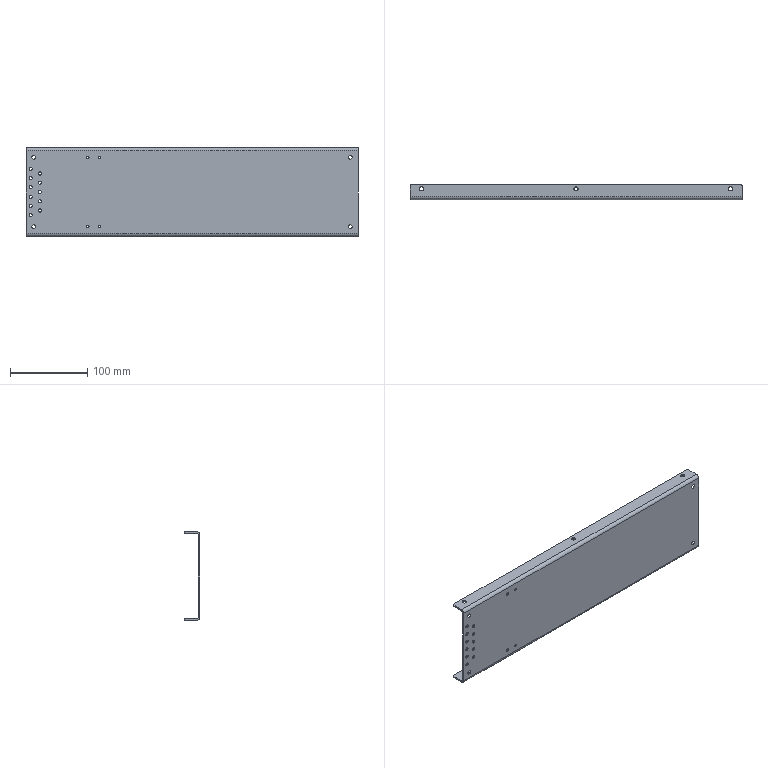Part | SolidWorks | features HoleWzd 4, EdgeFlange 1, Fillet 1, FlatPattern 1, SMBaseFlange 1, SheetMetal 1 | 1 solid | 76 faces | box 430 x 20 x 115 mm | volume 126667 mm3 | cylinder 50 | plane 18 | cone 8 | commonest cylinder face diameters 4.2 x22 5.5 x12 3.3 x8 4 x6 8 x2